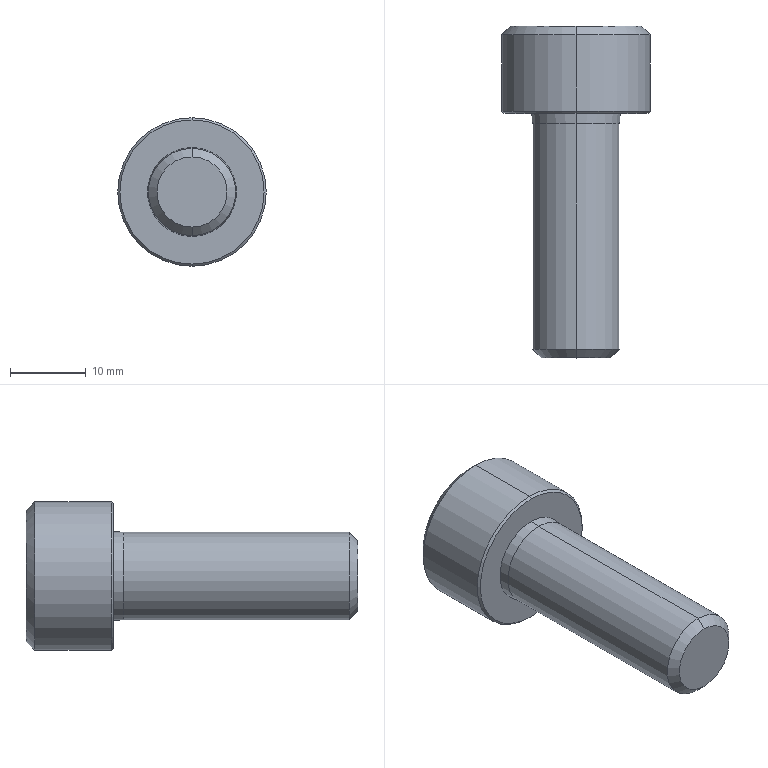Part | SolidWorks | features BaseBody 1 | 1 solid | 35 faces | box 19.615 x 43.846 x 19.615 mm | volume 6315 mm3 | cone 16 | plane 15 | cylinder 4 | commonest cylinder face diameters 11.538 x2 19.615 x2
STEP:
#1=CARTESIAN_POINT('',(-58.138,245.555,113.462));
#2=VERTEX_POINT('',#1);
#3=CARTESIAN_POINT('',(-58.138,245.555,101.923));
#4=VERTEX_POINT('',#3);
#5=CARTESIAN_POINT('',(-58.138,245.555,107.692));
#6=DIRECTION('',(0.,1.,0.));
#7=DIRECTION('',(0.,0.,1.));
#8=AXIS2_PLACEMENT_3D('',#5,#6,#7);
#9=CIRCLE('',#8,5.769);
#10=EDGE_CURVE('',#2,#4,#9,.T.);
#11=ORIENTED_EDGE('',*,*,#10,.T.);
#12=CARTESIAN_POINT('',(-58.138,275.346,101.923));
#13=VERTEX_POINT('',#12);
#14=CARTESIAN_POINT('',(-58.138,244.423,101.923));
#15=DIRECTION('',(0.,1.,0.));
#16=VECTOR('',#15,1000.);
#17=LINE('',#14,#16);
#18=EDGE_CURVE('',#4,#13,#17,.T.);
#19=ORIENTED_EDGE('',*,*,#18,.T.);
#20=CARTESIAN_POINT('',(-58.138,275.346,113.462));
#21=VERTEX_POINT('',#20);
#22=CARTESIAN_POINT('',(-58.138,275.346,107.692));
#23=DIRECTION('',(0.,-1.,0.));
#24=DIRECTION('',(0.,0.,1.));
#25=AXIS2_PLACEMENT_3D('',#22,#23,#24);
#26=CIRCLE('',#25,5.769);
#27=EDGE_CURVE('',#13,#21,#26,.T.);
#28=ORIENTED_EDGE('',*,*,#27,.T.);
#29=CARTESIAN_POINT('',(-58.138,244.423,113.462));
#30=DIRECTION('',(0.,1.,0.));
#31=VECTOR('',#30,1000.);
#32=LINE('',#29,#31);
#33=EDGE_CURVE('',#2,#21,#32,.T.);
#34=ORIENTED_EDGE('',*,*,#33,.F.);
#35=EDGE_LOOP('',(#11,#19,#28,#34));
#36=FACE_OUTER_BOUND('',#35,.T.);
#37=CARTESIAN_POINT('',(-58.138,244.423,107.692));
#38=DIRECTION('',(0.,1.,0.));
#39=DIRECTION('',(0.,0.,1.));
#40=AXIS2_PLACEMENT_3D('',#37,#38,#39);
#41=CYLINDRICAL_SURFACE('',#40,5.769);
#42=ADVANCED_FACE('',(#36),#41,.T.);
#43=ORIENTED_EDGE('',*,*,#27,.F.);
#44=CARTESIAN_POINT('',(-58.138,276.731,101.808));
#45=VERTEX_POINT('',#44);
#46=CARTESIAN_POINT('',(-58.138,276.731,101.808));
#47=DIRECTION('',(0.,0.9965,-0.08305));
#48=VECTOR('',#47,1000.);
#49=LINE('',#46,#48);
#50=EDGE_CURVE('',#13,#45,#49,.T.);
#51=ORIENTED_EDGE('',*,*,#50,.T.);
#52=CARTESIAN_POINT('',(-58.138,276.731,113.577));
#53=VERTEX_POINT('',#52);
#54=CARTESIAN_POINT('',(-58.138,276.731,107.692));
#55=DIRECTION('',(0.,-1.,0.));
#56=DIRECTION('',(0.,0.,1.));
#57=AXIS2_PLACEMENT_3D('',#54,#55,#56);
#58=CIRCLE('',#57,5.885);
#59=EDGE_CURVE('',#45,#53,#58,.T.);
#60=ORIENTED_EDGE('',*,*,#59,.T.);
#61=CARTESIAN_POINT('',(-58.138,276.731,113.577));
#62=DIRECTION('',(0.,0.9965,0.08305));
#63=VECTOR('',#62,1000.);
#64=LINE('',#61,#63);
#65=EDGE_CURVE('',#21,#53,#64,.T.);
#66=ORIENTED_EDGE('',*,*,#65,.F.);
#67=EDGE_LOOP('',(#43,#51,#60,#66));
#68=FACE_OUTER_BOUND('',#67,.T.);
#69=CARTESIAN_POINT('',(-58.138,276.731,107.692));
#70=DIRECTION('',(0.,1.,0.));
#71=DIRECTION('',(0.,0.,1.));
#72=AXIS2_PLACEMENT_3D('',#69,#70,#71);
#73=CONICAL_SURFACE('',#72,5.885,0.08314);
#74=ADVANCED_FACE('',(#68),#73,.T.);
#75=CARTESIAN_POINT('',(-58.138,244.423,112.33));
#76=VERTEX_POINT('',#75);
#77=CARTESIAN_POINT('',(-58.138,244.423,103.055));
#78=VERTEX_POINT('',#77);
#79=CARTESIAN_POINT('',(-58.138,244.423,107.692));
#80=DIRECTION('',(0.,1.,0.));
#81=DIRECTION('',(0.,0.,1.));
#82=AXIS2_PLACEMENT_3D('',#79,#80,#81);
#83=CIRCLE('',#82,4.637);
#84=EDGE_CURVE('',#76,#78,#83,.T.);
#85=ORIENTED_EDGE('',*,*,#84,.T.);
#86=CARTESIAN_POINT('',(-58.138,245.555,101.923));
#87=DIRECTION('',(0.,0.7071,-0.7071));
#88=VECTOR('',#87,1000.);
#89=LINE('',#86,#88);
#90=EDGE_CURVE('',#78,#4,#89,.T.);
#91=ORIENTED_EDGE('',*,*,#90,.T.);
#92=ORIENTED_EDGE('',*,*,#10,.F.);
#93=CARTESIAN_POINT('',(-58.138,245.555,113.462));
#94=DIRECTION('',(0.,0.7071,0.7071));
#95=VECTOR('',#94,1000.);
#96=LINE('',#93,#95);
#97=EDGE_CURVE('',#76,#2,#96,.T.);
#98=ORIENTED_EDGE('',*,*,#97,.F.);
#99=EDGE_LOOP('',(#85,#91,#92,#98));
#100=FACE_OUTER_BOUND('',#99,.T.);
#101=CARTESIAN_POINT('',(-58.138,245.555,107.692));
#102=DIRECTION('',(0.,1.,0.));
#103=DIRECTION('',(0.,0.,1.));
#104=AXIS2_PLACEMENT_3D('',#101,#102,#103);
#105=CONICAL_SURFACE('',#104,5.769,0.7854);
#106=ADVANCED_FACE('',(#100),#105,.T.);
#107=CARTESIAN_POINT('',(-58.138,276.731,117.212));
#108=VERTEX_POINT('',#107);
#109=CARTESIAN_POINT('',(-58.138,276.731,98.173));
#110=VERTEX_POINT('',#109);
#111=CARTESIAN_POINT('',(-58.138,276.731,107.692));
#112=DIRECTION('',(0.,1.,0.));
#113=DIRECTION('',(0.,0.,1.));
#114=AXIS2_PLACEMENT_3D('',#111,#112,#113);
#115=CIRCLE('',#114,9.519);
#116=EDGE_CURVE('',#108,#110,#115,.T.);
#117=ORIENTED_EDGE('',*,*,#116,.T.);
#118=CARTESIAN_POINT('',(-58.138,277.019,97.885));
#119=VERTEX_POINT('',#118);
#120=CARTESIAN_POINT('',(-58.138,277.019,97.885));
#121=DIRECTION('',(0.,0.7071,-0.7071));
#122=VECTOR('',#121,1000.);
#123=LINE('',#120,#122);
#124=EDGE_CURVE('',#110,#119,#123,.T.);
#125=ORIENTED_EDGE('',*,*,#124,.T.);
#126=CARTESIAN_POINT('',(-58.138,277.019,117.5));
#127=VERTEX_POINT('',#126);
#128=CARTESIAN_POINT('',(-58.138,277.019,107.692));
#129=DIRECTION('',(0.,-1.,0.));
#130=DIRECTION('',(-1.,0.,0.));
#131=AXIS2_PLACEMENT_3D('',#128,#129,#130);
#132=CIRCLE('',#131,9.808);
#133=EDGE_CURVE('',#119,#127,#132,.T.);
#134=ORIENTED_EDGE('',*,*,#133,.T.);
#135=CARTESIAN_POINT('',(-58.138,277.019,117.5));
#136=DIRECTION('',(0.,0.7071,0.7071));
#137=VECTOR('',#136,1000.);
#138=LINE('',#135,#137);
#139=EDGE_CURVE('',#108,#127,#138,.T.);
#140=ORIENTED_EDGE('',*,*,#139,.F.);
#141=EDGE_LOOP('',(#117,#125,#134,#140));
#142=FACE_OUTER_BOUND('',#141,.T.);
#143=CARTESIAN_POINT('',(-58.138,277.019,107.692));
#144=DIRECTION('',(0.,1.,0.));
#145=DIRECTION('',(0.,0.,1.));
#146=AXIS2_PLACEMENT_3D('',#143,#144,#145);
#147=CONICAL_SURFACE('',#146,9.808,0.7854);
#148=ADVANCED_FACE('',(#142),#147,.T.);
#149=ORIENTED_EDGE('',*,*,#133,.F.);
#150=CARTESIAN_POINT('',(-58.138,287.115,97.885));
#151=VERTEX_POINT('',#150);
#152=CARTESIAN_POINT('',(-58.138,244.423,97.885));
#153=DIRECTION('',(0.,1.,0.));
#154=VECTOR('',#153,1000.);
#155=LINE('',#152,#154);
#156=EDGE_CURVE('',#119,#151,#155,.T.);
#157=ORIENTED_EDGE('',*,*,#156,.T.);
#158=CARTESIAN_POINT('',(-58.138,287.115,117.5));
#159=VERTEX_POINT('',#158);
#160=CARTESIAN_POINT('',(-58.138,287.115,107.692));
#161=DIRECTION('',(0.,-1.,0.));
#162=DIRECTION('',(0.,0.,1.));
#163=AXIS2_PLACEMENT_3D('',#160,#161,#162);
#164=CIRCLE('',#163,9.808);
#165=EDGE_CURVE('',#151,#159,#164,.T.);
#166=ORIENTED_EDGE('',*,*,#165,.T.);
#167=CARTESIAN_POINT('',(-58.138,244.423,117.5));
#168=DIRECTION('',(0.,1.,0.));
#169=VECTOR('',#168,1000.);
#170=LINE('',#167,#169);
#171=EDGE_CURVE('',#127,#159,#170,.T.);
#172=ORIENTED_EDGE('',*,*,#171,.F.);
#173=EDGE_LOOP('',(#149,#157,#166,#172));
#174=FACE_OUTER_BOUND('',#173,.T.);
#175=CARTESIAN_POINT('',(-58.138,244.423,107.692));
#176=DIRECTION('',(0.,1.,0.));
#177=DIRECTION('',(0.,0.,1.));
#178=AXIS2_PLACEMENT_3D('',#175,#176,#177);
#179=CYLINDRICAL_SURFACE('',#178,9.808);
#180=ADVANCED_FACE('',(#174),#179,.T.);
#181=CARTESIAN_POINT('',(-58.138,288.269,99.038));
#182=VERTEX_POINT('',#181);
#183=CARTESIAN_POINT('',(-58.138,288.269,116.346));
#184=VERTEX_POINT('',#183);
#185=CARTESIAN_POINT('',(-58.138,288.269,107.692));
#186=DIRECTION('',(0.,-1.,0.));
#187=DIRECTION('',(0.,0.,-1.));
#188=AXIS2_PLACEMENT_3D('',#185,#186,#187);
#189=CIRCLE('',#188,8.654);
#190=EDGE_CURVE('',#182,#184,#189,.T.);
#191=ORIENTED_EDGE('',*,*,#190,.T.);
#192=CARTESIAN_POINT('',(-58.138,287.115,117.5));
#193=DIRECTION('',(0.,-0.7071,0.7071));
#194=VECTOR('',#193,1000.);
#195=LINE('',#192,#194);
#196=EDGE_CURVE('',#184,#159,#195,.T.);
#197=ORIENTED_EDGE('',*,*,#196,.T.);
#198=ORIENTED_EDGE('',*,*,#165,.F.);
#199=CARTESIAN_POINT('',(-58.138,287.115,97.885));
#200=DIRECTION('',(0.,-0.7071,-0.7071));
#201=VECTOR('',#200,1000.);
#202=LINE('',#199,#201);
#203=EDGE_CURVE('',#182,#151,#202,.T.);
#204=ORIENTED_EDGE('',*,*,#203,.F.);
#205=EDGE_LOOP('',(#191,#197,#198,#204));
#206=FACE_OUTER_BOUND('',#205,.T.);
#207=CARTESIAN_POINT('',(-58.138,287.115,107.692));
#208=DIRECTION('',(0.,-1.,0.));
#209=DIRECTION('',(0.,0.,-1.));
#210=AXIS2_PLACEMENT_3D('',#207,#208,#209);
#211=CONICAL_SURFACE('',#210,9.808,0.7854);
#212=ADVANCED_FACE('',(#206),#211,.T.);
#213=CARTESIAN_POINT('',(-58.138,279.835,107.692));
#214=VERTEX_POINT('',#213);
#215=CARTESIAN_POINT('',(-58.138,282.5,112.308));
#216=VERTEX_POINT('',#215);
#217=CARTESIAN_POINT('',(-58.138,282.5,112.308));
#218=DIRECTION('',(0.,0.5,0.866));
#219=VECTOR('',#218,1000.);
#220=LINE('',#217,#219);
#221=EDGE_CURVE('',#214,#216,#220,.T.);
#222=ORIENTED_EDGE('',*,*,#221,.F.);
#223=CARTESIAN_POINT('',(-58.138,282.5,103.077));
#224=VERTEX_POINT('',#223);
#225=CARTESIAN_POINT('',(-58.138,282.5,103.077));
#226=DIRECTION('',(0.,0.5,-0.866));
#227=VECTOR('',#226,1000.);
#228=LINE('',#225,#227);
#229=EDGE_CURVE('',#214,#224,#228,.T.);
#230=ORIENTED_EDGE('',*,*,#229,.T.);
#231=CARTESIAN_POINT('',(-60.446,282.5,103.695));
#232=VERTEX_POINT('',#231);
#233=CARTESIAN_POINT('',(-58.138,282.5,107.692));
#234=DIRECTION('',(0.,-1.,0.));
#235=DIRECTION('',(0.,0.,1.));
#236=AXIS2_PLACEMENT_3D('',#233,#234,#235);
#237=CIRCLE('',#236,4.615);
#238=EDGE_CURVE('',#232,#224,#237,.T.);
#239=ORIENTED_EDGE('',*,*,#238,.F.);
#240=CARTESIAN_POINT('',(-62.753,282.5,107.692));
#241=VERTEX_POINT('',#240);
#242=CARTESIAN_POINT('',(-58.138,282.5,107.692));
#243=DIRECTION('',(0.,-1.,0.));
#244=DIRECTION('',(0.,0.,1.));
#245=AXIS2_PLACEMENT_3D('',#242,#243,#244);
#246=CIRCLE('',#245,4.615);
#247=EDGE_CURVE('',#241,#232,#246,.T.);
#248=ORIENTED_EDGE('',*,*,#247,.F.);
#249=CARTESIAN_POINT('',(-60.446,282.5,111.689));
#250=VERTEX_POINT('',#249);
#251=CARTESIAN_POINT('',(-58.138,282.5,107.692));
#252=DIRECTION('',(0.,-1.,0.));
#253=DIRECTION('',(0.,0.,1.));
#254=AXIS2_PLACEMENT_3D('',#251,#252,#253);
#255=CIRCLE('',#254,4.615);
#256=EDGE_CURVE('',#250,#241,#255,.T.);
#257=ORIENTED_EDGE('',*,*,#256,.F.);
#258=CARTESIAN_POINT('',(-58.138,282.5,107.692));
#259=DIRECTION('',(0.,-1.,0.));
#260=DIRECTION('',(0.,0.,1.));
#261=AXIS2_PLACEMENT_3D('',#258,#259,#260);
#262=CIRCLE('',#261,4.615);
#263=EDGE_CURVE('',#216,#250,#262,.T.);
#264=ORIENTED_EDGE('',*,*,#263,.F.);
#265=EDGE_LOOP('',(#222,#230,#239,#248,#257,#264));
#266=FACE_OUTER_BOUND('',#265,.T.);
#267=CARTESIAN_POINT('',(-58.138,282.5,107.692));
#268=DIRECTION('',(0.,1.,0.));
#269=DIRECTION('',(0.,0.,1.));
#270=AXIS2_PLACEMENT_3D('',#267,#268,#269);
#271=CONICAL_SURFACE('',#270,4.615,1.047);
#272=ADVANCED_FACE('',(#266),#271,.F.);
#273=ORIENTED_EDGE('',*,*,#18,.F.);
#274=CARTESIAN_POINT('',(-58.138,245.555,107.692));
#275=DIRECTION('',(0.,1.,0.));
#276=DIRECTION('',(0.,0.,1.));
#277=AXIS2_PLACEMENT_3D('',#274,#275,#276);
#278=CIRCLE('',#277,5.769);
#279=EDGE_CURVE('',#4,#2,#278,.T.);
#280=ORIENTED_EDGE('',*,*,#279,.T.);
#281=ORIENTED_EDGE('',*,*,#33,.T.);
#282=CARTESIAN_POINT('',(-58.138,275.346,107.692));
#283=DIRECTION('',(0.,-1.,0.));
#284=DIRECTION('',(0.,0.,1.));
#285=AXIS2_PLACEMENT_3D('',#282,#283,#284);
#286=CIRCLE('',#285,5.769);
#287=EDGE_CURVE('',#21,#13,#286,.T.);
#288=ORIENTED_EDGE('',*,*,#287,.T.);
#289=EDGE_LOOP('',(#273,#280,#281,#288));
#290=FACE_OUTER_BOUND('',#289,.T.);
#291=CARTESIAN_POINT('',(-58.138,244.423,107.692));
#292=DIRECTION('',(0.,1.,0.));
#293=DIRECTION('',(0.,0.,1.));
#294=AXIS2_PLACEMENT_3D('',#291,#292,#293);
#295=CYLINDRICAL_SURFACE('',#294,5.769);
#296=ADVANCED_FACE('',(#290),#295,.T.);
#297=ORIENTED_EDGE('',*,*,#50,.F.);
#298=ORIENTED_EDGE('',*,*,#287,.F.);
#299=ORIENTED_EDGE('',*,*,#65,.T.);
#300=CARTESIAN_POINT('',(-58.138,276.731,107.692));
#301=DIRECTION('',(0.,-1.,0.));
#302=DIRECTION('',(0.,0.,1.));
#303=AXIS2_PLACEMENT_3D('',#300,#301,#302);
#304=CIRCLE('',#303,5.885);
#305=EDGE_CURVE('',#53,#45,#304,.T.);
#306=ORIENTED_EDGE('',*,*,#305,.T.);
#307=EDGE_LOOP('',(#297,#298,#299,#306));
#308=FACE_OUTER_BOUND('',#307,.T.);
#309=CARTESIAN_POINT('',(-58.138,276.731,107.692));
#310=DIRECTION('',(0.,1.,0.));
#311=DIRECTION('',(0.,0.,1.));
#312=AXIS2_PLACEMENT_3D('',#309,#310,#311);
#313=CONICAL_SURFACE('',#312,5.885,0.08314);
#314=ADVANCED_FACE('',(#308),#313,.T.);
#315=ORIENTED_EDGE('',*,*,#90,.F.);
#316=CARTESIAN_POINT('',(-58.138,244.423,107.692));
#317=DIRECTION('',(0.,1.,0.));
#318=DIRECTION('',(0.,0.,1.));
#319=AXIS2_PLACEMENT_3D('',#316,#317,#318);
#320=CIRCLE('',#319,4.637);
#321=EDGE_CURVE('',#78,#76,#320,.T.);
#322=ORIENTED_EDGE('',*,*,#321,.T.);
#323=ORIENTED_EDGE('',*,*,#97,.T.);
#324=ORIENTED_EDGE('',*,*,#279,.F.);
#325=EDGE_LOOP('',(#315,#322,#323,#324));
#326=FACE_OUTER_BOUND('',#325,.T.);
#327=CARTESIAN_POINT('',(-58.138,245.555,107.692));
#328=DIRECTION('',(0.,1.,0.));
#329=DIRECTION('',(0.,0.,1.));
#330=AXIS2_PLACEMENT_3D('',#327,#328,#329);
#331=CONICAL_SURFACE('',#330,5.769,0.7854);
#332=ADVANCED_FACE('',(#326),#331,.T.);
#333=ORIENTED_EDGE('',*,*,#305,.F.);
#334=ORIENTED_EDGE('',*,*,#59,.F.);
#335=EDGE_LOOP('',(#333,#334));
#336=FACE_BOUND('',#335,.T.);
#337=ORIENTED_EDGE('',*,*,#116,.F.);
#338=CARTESIAN_POINT('',(-58.138,276.731,107.692));
#339=DIRECTION('',(0.,1.,0.));
#340=DIRECTION('',(0.,0.,1.));
#341=AXIS2_PLACEMENT_3D('',#338,#339,#340);
#342=CIRCLE('',#341,9.519);
#343=EDGE_CURVE('',#110,#108,#342,.T.);
#344=ORIENTED_EDGE('',*,*,#343,.F.);
#345=EDGE_LOOP('',(#337,#344));
#346=FACE_OUTER_BOUND('',#345,.T.);
#347=CARTESIAN_POINT('',(-67.657,276.731,107.692));
#348=DIRECTION('',(0.,1.,0.));
#349=DIRECTION('',(0.,0.,1.));
#350=AXIS2_PLACEMENT_3D('',#347,#348,#349);
#351=PLANE('',#350);
#352=ADVANCED_FACE('',(#336,#346),#351,.F.);
#353=ORIENTED_EDGE('',*,*,#84,.F.);
#354=ORIENTED_EDGE('',*,*,#321,.F.);
#355=EDGE_LOOP('',(#353,#354));
#356=FACE_OUTER_BOUND('',#355,.T.);
#357=CARTESIAN_POINT('',(-62.775,244.423,107.692));
#358=DIRECTION('',(0.,1.,0.));
#359=DIRECTION('',(0.,0.,1.));
#360=AXIS2_PLACEMENT_3D('',#357,#358,#359);
#361=PLANE('',#360);
#362=ADVANCED_FACE('',(#356),#361,.F.);
#363=ORIENTED_EDGE('',*,*,#124,.F.);
#364=ORIENTED_EDGE('',*,*,#343,.T.);
#365=ORIENTED_EDGE('',*,*,#139,.T.);
#366=CARTESIAN_POINT('',(-58.138,277.019,107.692));
#367=DIRECTION('',(0.,-1.,0.));
#368=DIRECTION('',(-1.,0.,0.));
#369=AXIS2_PLACEMENT_3D('',#366,#367,#368);
#370=CIRCLE('',#369,9.808);
#371=EDGE_CURVE('',#127,#119,#370,.T.);
#372=ORIENTED_EDGE('',*,*,#371,.T.);
#373=EDGE_LOOP('',(#363,#364,#365,#372));
#374=FACE_OUTER_BOUND('',#373,.T.);
#375=CARTESIAN_POINT('',(-58.138,277.019,107.692));
#376=DIRECTION('',(0.,1.,0.));
#377=DIRECTION('',(0.,0.,1.));
#378=AXIS2_PLACEMENT_3D('',#375,#376,#377);
#379=CONICAL_SURFACE('',#378,9.808,0.7854);
#380=ADVANCED_FACE('',(#374),#379,.T.);
#381=ORIENTED_EDGE('',*,*,#156,.F.);
#382=ORIENTED_EDGE('',*,*,#371,.F.);
#383=ORIENTED_EDGE('',*,*,#171,.T.);
#384=CARTESIAN_POINT('',(-58.138,287.115,107.692));
#385=DIRECTION('',(0.,-1.,0.));
#386=DIRECTION('',(0.,0.,1.));
#387=AXIS2_PLACEMENT_3D('',#384,#385,#386);
#388=CIRCLE('',#387,9.808);
#389=EDGE_CURVE('',#159,#151,#388,.T.);
#390=ORIENTED_EDGE('',*,*,#389,.T.);
#391=EDGE_LOOP('',(#381,#382,#383,#390));
#392=FACE_OUTER_BOUND('',#391,.T.);
#393=CARTESIAN_POINT('',(-58.138,244.423,107.692));
#394=DIRECTION('',(0.,1.,0.));
#395=DIRECTION('',(0.,0.,1.));
#396=AXIS2_PLACEMENT_3D('',#393,#394,#395);
#397=CYLINDRICAL_SURFACE('',#396,9.808);
#398=ADVANCED_FACE('',(#392),#397,.T.);
#399=ORIENTED_EDGE('',*,*,#196,.F.);
#400=CARTESIAN_POINT('',(-58.138,288.269,107.692));
#401=DIRECTION('',(0.,-1.,0.));
#402=DIRECTION('',(0.,0.,-1.));
#403=AXIS2_PLACEMENT_3D('',#400,#401,#402);
#404=CIRCLE('',#403,8.654);
#405=EDGE_CURVE('',#184,#182,#404,.T.);
#406=ORIENTED_EDGE('',*,*,#405,.T.);
#407=ORIENTED_EDGE('',*,*,#203,.T.);
#408=ORIENTED_EDGE('',*,*,#389,.F.);
#409=EDGE_LOOP('',(#399,#406,#407,#408));
#410=FACE_OUTER_BOUND('',#409,.T.);
#411=CARTESIAN_POINT('',(-58.138,287.115,107.692));
#412=DIRECTION('',(0.,-1.,0.));
#413=DIRECTION('',(0.,0.,-1.));
#414=AXIS2_PLACEMENT_3D('',#411,#412,#413);
#415=CONICAL_SURFACE('',#414,9.808,0.7854);
#416=ADVANCED_FACE('',(#410),#415,.T.);
#417=CARTESIAN_POINT('',(-53.523,288.269,105.028));
#418=VERTEX_POINT('',#417);
#419=CARTESIAN_POINT('',(-58.138,288.269,102.363));
#420=VERTEX_POINT('',#419);
#421=CARTESIAN_POINT('',(-58.138,288.269,107.692));
#422=DIRECTION('',(0.,1.,0.));
#423=DIRECTION('',(0.,0.,1.));
#424=AXIS2_PLACEMENT_3D('',#421,#422,#423);
#425=CIRCLE('',#424,5.329);
#426=EDGE_CURVE('',#418,#420,#425,.T.);
#427=ORIENTED_EDGE('',*,*,#426,.F.);
#428=CARTESIAN_POINT('',(-53.523,288.269,110.357));
#429=VERTEX_POINT('',#428);
#430=CARTESIAN_POINT('',(-58.138,288.269,107.692));
#431=DIRECTION('',(0.,1.,0.));
#432=DIRECTION('',(0.,0.,1.));
#433=AXIS2_PLACEMENT_3D('',#430,#431,#432);
#434=CIRCLE('',#433,5.329);
#435=EDGE_CURVE('',#429,#418,#434,.T.);
#436=ORIENTED_EDGE('',*,*,#435,.F.);
#437=CARTESIAN_POINT('',(-58.138,288.269,113.022));
#438=VERTEX_POINT('',#437);
#439=CARTESIAN_POINT('',(-58.138,288.269,107.692));
#440=DIRECTION('',(0.,1.,0.));
#441=DIRECTION('',(0.,0.,1.));
#442=AXIS2_PLACEMENT_3D('',#439,#440,#441);
#443=CIRCLE('',#442,5.329);
#444=EDGE_CURVE('',#438,#429,#443,.T.);
#445=ORIENTED_EDGE('',*,*,#444,.F.);
#446=CARTESIAN_POINT('',(-62.753,288.269,110.357));
#447=VERTEX_POINT('',#446);
#448=CARTESIAN_POINT('',(-58.138,288.269,107.692));
#449=DIRECTION('',(0.,1.,0.));
#450=DIRECTION('',(0.,0.,1.));
#451=AXIS2_PLACEMENT_3D('',#448,#449,#450);
#452=CIRCLE('',#451,5.329);
#453=EDGE_CURVE('',#447,#438,#452,.T.);
#454=ORIENTED_EDGE('',*,*,#453,.F.);
#455=CARTESIAN_POINT('',(-62.753,288.269,105.028));
#456=VERTEX_POINT('',#455);
#457=CARTESIAN_POINT('',(-58.138,288.269,107.692));
#458=DIRECTION('',(0.,1.,0.));
#459=DIRECTION('',(0.,0.,1.));
#460=AXIS2_PLACEMENT_3D('',#457,#458,#459);
#461=CIRCLE('',#460,5.329);
#462=EDGE_CURVE('',#456,#447,#461,.T.);
#463=ORIENTED_EDGE('',*,*,#462,.F.);
#464=CARTESIAN_POINT('',(-58.138,288.269,107.692));
#465=DIRECTION('',(0.,1.,0.));
#466=DIRECTION('',(0.,0.,1.));
#467=AXIS2_PLACEMENT_3D('',#464,#465,#466);
#468=CIRCLE('',#467,5.329);
#469=EDGE_CURVE('',#420,#456,#468,.T.);
#470=ORIENTED_EDGE('',*,*,#469,.F.);
#471=EDGE_LOOP('',(#427,#436,#445,#454,#463,#470));
#472=FACE_BOUND('',#471,.T.);
#473=ORIENTED_EDGE('',*,*,#190,.F.);
#474=ORIENTED_EDGE('',*,*,#405,.F.);
#475=EDGE_LOOP('',(#473,#474));
#476=FACE_OUTER_BOUND('',#475,.T.);
#477=CARTESIAN_POINT('',(-63.467,288.269,107.692));
#478=DIRECTION('',(0.,-1.,0.));
#479=DIRECTION('',(0.,0.,-1.));
#480=AXIS2_PLACEMENT_3D('',#477,#478,#479);
#481=PLANE('',#480);
#482=ADVANCED_FACE('',(#472,#476),#481,.F.);
#483=CARTESIAN_POINT('',(-58.138,288.269,102.363));
#484=CARTESIAN_POINT('',(-58.499,288.061,102.571));
#485=CARTESIAN_POINT('',(-58.867,287.884,102.784));
#486=CARTESIAN_POINT('',(-59.44,287.694,103.115));
#487=CARTESIAN_POINT('',(-59.635,287.644,103.227));
#488=CARTESIAN_POINT('',(-60.031,287.574,103.456));
#489=CARTESIAN_POINT('',(-60.236,287.556,103.574));
#490=CARTESIAN_POINT('',(-60.84,287.554,103.923));
#491=CARTESIAN_POINT('',(-61.236,287.625,104.152));
#492=CARTESIAN_POINT('',(-62.017,287.88,104.603));
#493=CARTESIAN_POINT('',(-62.391,288.06,104.818));
#494=CARTESIAN_POINT('',(-62.753,288.269,105.028));
#495=B_SPLINE_CURVE_WITH_KNOTS('',3,(#483,#484,#485,#486,#487,#488,#489,#490,#491,#492,#493,#494),.UNSPECIFIED.,.F.,.F.,(4,2,2,2,2,4),(0.,0.001376,0.002064,0.002753,0.004129,0.005505),.UNSPECIFIED.);
#496=EDGE_CURVE('',#420,#456,#495,.T.);
#497=ORIENTED_EDGE('',*,*,#496,.F.);
#498=ORIENTED_EDGE('',*,*,#469,.T.);
#499=EDGE_LOOP('',(#497,#498));
#500=FACE_OUTER_BOUND('',#499,.T.);
#501=CARTESIAN_POINT('',(-58.138,288.269,107.692));
#502=DIRECTION('',(0.,1.,0.));
#503=DIRECTION('',(0.,0.,1.));
#504=AXIS2_PLACEMENT_3D('',#501,#502,#503);
#505=CONICAL_SURFACE('',#504,5.329,0.7854);
#506=ADVANCED_FACE('',(#500),#505,.F.);
#507=CARTESIAN_POINT('',(-53.523,288.269,105.028));
#508=CARTESIAN_POINT('',(-53.883,288.061,104.819));
#509=CARTESIAN_POINT('',(-54.252,287.884,104.607));
#510=CARTESIAN_POINT('',(-54.825,287.694,104.276));
#511=CARTESIAN_POINT('',(-55.019,287.644,104.164));
#512=CARTESIAN_POINT('',(-55.416,287.574,103.934));
#513=CARTESIAN_POINT('',(-55.62,287.556,103.816));
#514=CARTESIAN_POINT('',(-56.225,287.554,103.468));
#515=CARTESIAN_POINT('',(-56.621,287.625,103.239));
#516=CARTESIAN_POINT('',(-57.402,287.88,102.788));
#517=CARTESIAN_POINT('',(-57.775,288.06,102.572));
#518=CARTESIAN_POINT('',(-58.138,288.269,102.363));
#519=B_SPLINE_CURVE_WITH_KNOTS('',3,(#507,#508,#509,#510,#511,#512,#513,#514,#515,#516,#517,#518),.UNSPECIFIED.,.F.,.F.,(4,2,2,2,2,4),(0.,0.001376,0.002064,0.002753,0.004129,0.005505),.UNSPECIFIED.);
#520=EDGE_CURVE('',#418,#420,#519,.T.);
#521=ORIENTED_EDGE('',*,*,#520,.F.);
#522=ORIENTED_EDGE('',*,*,#426,.T.);
#523=EDGE_LOOP('',(#521,#522));
#524=FACE_OUTER_BOUND('',#523,.T.);
#525=CARTESIAN_POINT('',(-58.138,288.269,107.692));
#526=DIRECTION('',(0.,1.,0.));
#527=DIRECTION('',(0.,0.,1.));
#528=AXIS2_PLACEMENT_3D('',#525,#526,#527);
#529=CONICAL_SURFACE('',#528,5.329,0.7854);
#530=ADVANCED_FACE('',(#524),#529,.F.);
#531=CARTESIAN_POINT('',(-53.523,288.269,110.357));
#532=CARTESIAN_POINT('',(-53.523,288.061,109.941));
#533=CARTESIAN_POINT('',(-53.523,287.884,109.515));
#534=CARTESIAN_POINT('',(-53.523,287.694,108.853));
#535=CARTESIAN_POINT('',(-53.523,287.644,108.629));
#536=CARTESIAN_POINT('',(-53.523,287.574,108.171));
#537=CARTESIAN_POINT('',(-53.523,287.556,107.935));
#538=CARTESIAN_POINT('',(-53.523,287.554,107.237));
#539=CARTESIAN_POINT('',(-53.523,287.625,106.78));
#540=CARTESIAN_POINT('',(-53.523,287.88,105.878));
#541=CARTESIAN_POINT('',(-53.523,288.06,105.446));
#542=CARTESIAN_POINT('',(-53.523,288.269,105.028));
#543=B_SPLINE_CURVE_WITH_KNOTS('',3,(#531,#532,#533,#534,#535,#536,#537,#538,#539,#540,#541,#542),.UNSPECIFIED.,.F.,.F.,(4,2,2,2,2,4),(0.,0.001376,0.002064,0.002753,0.004129,0.005505),.UNSPECIFIED.);
#544=EDGE_CURVE('',#429,#418,#543,.T.);
#545=ORIENTED_EDGE('',*,*,#544,.F.);
#546=ORIENTED_EDGE('',*,*,#435,.T.);
#547=EDGE_LOOP('',(#545,#546));
#548=FACE_OUTER_BOUND('',#547,.T.);
#549=CARTESIAN_POINT('',(-58.138,288.269,107.692));
#550=DIRECTION('',(0.,1.,0.));
#551=DIRECTION('',(0.,0.,1.));
#552=AXIS2_PLACEMENT_3D('',#549,#550,#551);
#553=CONICAL_SURFACE('',#552,5.329,0.7854);
#554=ADVANCED_FACE('',(#548),#553,.F.);
#555=CARTESIAN_POINT('',(-58.138,288.269,113.022));
#556=CARTESIAN_POINT('',(-57.777,288.061,112.813));
#557=CARTESIAN_POINT('',(-57.409,287.884,112.601));
#558=CARTESIAN_POINT('',(-56.836,287.694,112.27));
#559=CARTESIAN_POINT('',(-56.642,287.644,112.158));
#560=CARTESIAN_POINT('',(-56.245,287.574,111.929));
#561=CARTESIAN_POINT('',(-56.04,287.556,111.811));
#562=CARTESIAN_POINT('',(-55.436,287.554,111.462));
#563=CARTESIAN_POINT('',(-55.04,287.625,111.233));
#564=CARTESIAN_POINT('',(-54.259,287.88,110.782));
#565=CARTESIAN_POINT('',(-53.885,288.06,110.566));
#566=CARTESIAN_POINT('',(-53.523,288.269,110.357));
#567=B_SPLINE_CURVE_WITH_KNOTS('',3,(#555,#556,#557,#558,#559,#560,#561,#562,#563,#564,#565,#566),.UNSPECIFIED.,.F.,.F.,(4,2,2,2,2,4),(0.,0.001376,0.002064,0.002753,0.004129,0.005505),.UNSPECIFIED.);
#568=EDGE_CURVE('',#438,#429,#567,.T.);
#569=ORIENTED_EDGE('',*,*,#568,.F.);
#570=ORIENTED_EDGE('',*,*,#444,.T.);
#571=EDGE_LOOP('',(#569,#570));
#572=FACE_OUTER_BOUND('',#571,.T.);
#573=CARTESIAN_POINT('',(-58.138,288.269,107.692));
#574=DIRECTION('',(0.,1.,0.));
#575=DIRECTION('',(0.,0.,1.));
#576=AXIS2_PLACEMENT_3D('',#573,#574,#575);
#577=CONICAL_SURFACE('',#576,5.329,0.7854);
#578=ADVANCED_FACE('',(#572),#577,.F.);
#579=CARTESIAN_POINT('',(-62.753,288.269,110.357));
#580=CARTESIAN_POINT('',(-62.393,288.061,110.565));
#581=CARTESIAN_POINT('',(-62.024,287.884,110.778));
#582=CARTESIAN_POINT('',(-61.451,287.694,111.109));
#583=CARTESIAN_POINT('',(-61.257,287.644,111.221));
#584=CARTESIAN_POINT('',(-60.86,287.574,111.45));
#585=CARTESIAN_POINT('',(-60.656,287.556,111.568));
#586=CARTESIAN_POINT('',(-60.051,287.554,111.917));
#587=CARTESIAN_POINT('',(-59.655,287.625,112.146));
#588=CARTESIAN_POINT('',(-58.874,287.88,112.597));
#589=CARTESIAN_POINT('',(-58.501,288.06,112.812));
#590=CARTESIAN_POINT('',(-58.138,288.269,113.022));
#591=B_SPLINE_CURVE_WITH_KNOTS('',3,(#579,#580,#581,#582,#583,#584,#585,#586,#587,#588,#589,#590),.UNSPECIFIED.,.F.,.F.,(4,2,2,2,2,4),(0.,0.001376,0.002064,0.002753,0.004129,0.005505),.UNSPECIFIED.);
#592=EDGE_CURVE('',#447,#438,#591,.T.);
#593=ORIENTED_EDGE('',*,*,#592,.F.);
#594=ORIENTED_EDGE('',*,*,#453,.T.);
#595=EDGE_LOOP('',(#593,#594));
#596=FACE_OUTER_BOUND('',#595,.T.);
#597=CARTESIAN_POINT('',(-58.138,288.269,107.692));
#598=DIRECTION('',(0.,1.,0.));
#599=DIRECTION('',(0.,0.,1.));
#600=AXIS2_PLACEMENT_3D('',#597,#598,#599);
#601=CONICAL_SURFACE('',#600,5.329,0.7854);
#602=ADVANCED_FACE('',(#596),#601,.F.);
#603=CARTESIAN_POINT('',(-62.753,288.269,105.028));
#604=CARTESIAN_POINT('',(-62.753,288.061,105.444));
#605=CARTESIAN_POINT('',(-62.753,287.884,105.87));
#606=CARTESIAN_POINT('',(-62.753,287.694,106.531));
#607=CARTESIAN_POINT('',(-62.753,287.644,106.756));
#608=CARTESIAN_POINT('',(-62.753,287.574,107.214));
#609=CARTESIAN_POINT('',(-62.753,287.556,107.45));
#610=CARTESIAN_POINT('',(-62.753,287.554,108.148));
#611=CARTESIAN_POINT('',(-62.753,287.625,108.605));
#612=CARTESIAN_POINT('',(-62.753,287.88,109.507));
#613=CARTESIAN_POINT('',(-62.753,288.06,109.938));
#614=CARTESIAN_POINT('',(-62.753,288.269,110.357));
#615=B_SPLINE_CURVE_WITH_KNOTS('',3,(#603,#604,#605,#606,#607,#608,#609,#610,#611,#612,#613,#614),.UNSPECIFIED.,.F.,.F.,(4,2,2,2,2,4),(0.,0.001376,0.002064,0.002753,0.004129,0.005505),.UNSPECIFIED.);
#616=EDGE_CURVE('',#456,#447,#615,.T.);
#617=ORIENTED_EDGE('',*,*,#616,.F.);
#618=ORIENTED_EDGE('',*,*,#462,.T.);
#619=EDGE_LOOP('',(#617,#618));
#620=FACE_OUTER_BOUND('',#619,.T.);
#621=CARTESIAN_POINT('',(-58.138,288.269,107.692));
#622=DIRECTION('',(0.,1.,0.));
#623=DIRECTION('',(0.,0.,1.));
#624=AXIS2_PLACEMENT_3D('',#621,#622,#623);
#625=CONICAL_SURFACE('',#624,5.329,0.7854);
#626=ADVANCED_FACE('',(#620),#625,.F.);
#627=CARTESIAN_POINT('',(-62.753,282.5,105.028));
#628=VERTEX_POINT('',#627);
#629=CARTESIAN_POINT('',(-62.753,282.5,105.028));
#630=DIRECTION('',(0.,1.,0.));
#631=VECTOR('',#630,1000.);
#632=LINE('',#629,#631);
#633=EDGE_CURVE('',#628,#456,#632,.T.);
#634=ORIENTED_EDGE('',*,*,#633,.F.);
#635=CARTESIAN_POINT('',(-58.138,282.5,102.363));
#636=DIRECTION('',(-0.866,0.,0.5));
#637=VECTOR('',#636,1000.);
#638=LINE('',#635,#637);
#639=EDGE_CURVE('',#232,#628,#638,.T.);
#640=ORIENTED_EDGE('',*,*,#639,.F.);
#641=CARTESIAN_POINT('',(-58.138,282.5,102.363));
#642=VERTEX_POINT('',#641);
#643=CARTESIAN_POINT('',(-58.138,282.5,102.363));
#644=DIRECTION('',(-0.866,0.,0.5));
#645=VECTOR('',#644,1000.);
#646=LINE('',#643,#645);
#647=EDGE_CURVE('',#642,#232,#646,.T.);
#648=ORIENTED_EDGE('',*,*,#647,.F.);
#649=CARTESIAN_POINT('',(-58.138,282.5,102.363));
#650=DIRECTION('',(0.,-1.,0.));
#651=VECTOR('',#650,1000.);
#652=LINE('',#649,#651);
#653=EDGE_CURVE('',#420,#642,#652,.T.);
#654=ORIENTED_EDGE('',*,*,#653,.F.);
#655=ORIENTED_EDGE('',*,*,#496,.T.);
#656=EDGE_LOOP('',(#634,#640,#648,#654,#655));
#657=FACE_OUTER_BOUND('',#656,.T.);
#658=CARTESIAN_POINT('',(-58.138,282.5,102.363));
#659=DIRECTION('',(-0.5,0.,-0.866));
#660=DIRECTION('',(-0.866,0.,0.5));
#661=AXIS2_PLACEMENT_3D('',#658,#659,#660);
#662=PLANE('',#661);
#663=ADVANCED_FACE('',(#657),#662,.F.);
#664=ORIENTED_EDGE('',*,*,#653,.T.);
#665=CARTESIAN_POINT('',(-55.83,282.5,103.695));
#666=VERTEX_POINT('',#665);
#667=CARTESIAN_POINT('',(-53.523,282.5,105.028));
#668=DIRECTION('',(-0.866,0.,-0.5));
#669=VECTOR('',#668,1000.);
#670=LINE('',#667,#669);
#671=EDGE_CURVE('',#666,#642,#670,.T.);
#672=ORIENTED_EDGE('',*,*,#671,.F.);
#673=CARTESIAN_POINT('',(-53.523,282.5,105.028));
#674=VERTEX_POINT('',#673);
#675=CARTESIAN_POINT('',(-53.523,282.5,105.028));
#676=DIRECTION('',(-0.866,0.,-0.5));
#677=VECTOR('',#676,1000.);
#678=LINE('',#675,#677);
#679=EDGE_CURVE('',#674,#666,#678,.T.);
#680=ORIENTED_EDGE('',*,*,#679,.F.);
#681=CARTESIAN_POINT('',(-53.523,282.5,105.028));
#682=DIRECTION('',(0.,-1.,0.));
#683=VECTOR('',#682,1000.);
#684=LINE('',#681,#683);
#685=EDGE_CURVE('',#418,#674,#684,.T.);
#686=ORIENTED_EDGE('',*,*,#685,.F.);
#687=ORIENTED_EDGE('',*,*,#520,.T.);
#688=EDGE_LOOP('',(#664,#672,#680,#686,#687));
#689=FACE_OUTER_BOUND('',#688,.T.);
#690=CARTESIAN_POINT('',(-53.523,282.5,105.028));
#691=DIRECTION('',(0.5,0.,-0.866));
#692=DIRECTION('',(-0.866,0.,-0.5));
#693=AXIS2_PLACEMENT_3D('',#690,#691,#692);
#694=PLANE('',#693);
#695=ADVANCED_FACE('',(#689),#694,.F.);
#696=ORIENTED_EDGE('',*,*,#685,.T.);
#697=CARTESIAN_POINT('',(-53.523,282.5,107.692));
#698=VERTEX_POINT('',#697);
#699=CARTESIAN_POINT('',(-53.523,282.5,110.357));
#700=DIRECTION('',(0.,0.,-1.));
#701=VECTOR('',#700,1000.);
#702=LINE('',#699,#701);
#703=EDGE_CURVE('',#698,#674,#702,.T.);
#704=ORIENTED_EDGE('',*,*,#703,.F.);
#705=CARTESIAN_POINT('',(-53.523,282.5,110.357));
#706=VERTEX_POINT('',#705);
#707=CARTESIAN_POINT('',(-53.523,282.5,110.357));
#708=DIRECTION('',(0.,0.,-1.));
#709=VECTOR('',#708,1000.);
#710=LINE('',#707,#709);
#711=EDGE_CURVE('',#706,#698,#710,.T.);
#712=ORIENTED_EDGE('',*,*,#711,.F.);
#713=CARTESIAN_POINT('',(-53.523,282.5,110.357));
#714=DIRECTION('',(0.,-1.,0.));
#715=VECTOR('',#714,1000.);
#716=LINE('',#713,#715);
#717=EDGE_CURVE('',#429,#706,#716,.T.);
#718=ORIENTED_EDGE('',*,*,#717,.F.);
#719=ORIENTED_EDGE('',*,*,#544,.T.);
#720=EDGE_LOOP('',(#696,#704,#712,#718,#719));
#721=FACE_OUTER_BOUND('',#720,.T.);
#722=CARTESIAN_POINT('',(-53.523,282.5,110.357));
#723=DIRECTION('',(1.,0.,0.));
#724=DIRECTION('',(0.,0.,-1.));
#725=AXIS2_PLACEMENT_3D('',#722,#723,#724);
#726=PLANE('',#725);
#727=ADVANCED_FACE('',(#721),#726,.F.);
#728=ORIENTED_EDGE('',*,*,#717,.T.);
#729=CARTESIAN_POINT('',(-55.83,282.5,111.689));
#730=VERTEX_POINT('',#729);
#731=CARTESIAN_POINT('',(-58.138,282.5,113.022));
#732=DIRECTION('',(0.866,0.,-0.5));
#733=VECTOR('',#732,1000.);
#734=LINE('',#731,#733);
#735=EDGE_CURVE('',#730,#706,#734,.T.);
#736=ORIENTED_EDGE('',*,*,#735,.F.);
#737=CARTESIAN_POINT('',(-58.138,282.5,113.022));
#738=VERTEX_POINT('',#737);
#739=CARTESIAN_POINT('',(-58.138,282.5,113.022));
#740=DIRECTION('',(0.866,0.,-0.5));
#741=VECTOR('',#740,1000.);
#742=LINE('',#739,#741);
#743=EDGE_CURVE('',#738,#730,#742,.T.);
#744=ORIENTED_EDGE('',*,*,#743,.F.);
#745=CARTESIAN_POINT('',(-58.138,282.5,113.022));
#746=DIRECTION('',(0.,-1.,0.));
#747=VECTOR('',#746,1000.);
#748=LINE('',#745,#747);
#749=EDGE_CURVE('',#438,#738,#748,.T.);
#750=ORIENTED_EDGE('',*,*,#749,.F.);
#751=ORIENTED_EDGE('',*,*,#568,.T.);
#752=EDGE_LOOP('',(#728,#736,#744,#750,#751));
#753=FACE_OUTER_BOUND('',#752,.T.);
#754=CARTESIAN_POINT('',(-58.138,282.5,113.022));
#755=DIRECTION('',(0.5,0.,0.866));
#756=DIRECTION('',(0.866,0.,-0.5));
#757=AXIS2_PLACEMENT_3D('',#754,#755,#756);
#758=PLANE('',#757);
#759=ADVANCED_FACE('',(#753),#758,.F.);
#760=ORIENTED_EDGE('',*,*,#749,.T.);
#761=CARTESIAN_POINT('',(-62.753,282.5,110.357));
#762=DIRECTION('',(0.866,0.,0.5));
#763=VECTOR('',#762,1000.);
#764=LINE('',#761,#763);
#765=EDGE_CURVE('',#250,#738,#764,.T.);
#766=ORIENTED_EDGE('',*,*,#765,.F.);
#767=CARTESIAN_POINT('',(-62.753,282.5,110.357));
#768=VERTEX_POINT('',#767);
#769=CARTESIAN_POINT('',(-62.753,282.5,110.357));
#770=DIRECTION('',(0.866,0.,0.5));
#771=VECTOR('',#770,1000.);
#772=LINE('',#769,#771);
#773=EDGE_CURVE('',#768,#250,#772,.T.);
#774=ORIENTED_EDGE('',*,*,#773,.F.);
#775=CARTESIAN_POINT('',(-62.753,282.5,110.357));
#776=DIRECTION('',(0.,-1.,0.));
#777=VECTOR('',#776,1000.);
#778=LINE('',#775,#777);
#779=EDGE_CURVE('',#447,#768,#778,.T.);
#780=ORIENTED_EDGE('',*,*,#779,.F.);
#781=ORIENTED_EDGE('',*,*,#592,.T.);
#782=EDGE_LOOP('',(#760,#766,#774,#780,#781));
#783=FACE_OUTER_BOUND('',#782,.T.);
#784=CARTESIAN_POINT('',(-62.753,282.5,110.357));
#785=DIRECTION('',(-0.5,0.,0.866));
#786=DIRECTION('',(0.866,0.,0.5));
#787=AXIS2_PLACEMENT_3D('',#784,#785,#786);
#788=PLANE('',#787);
#789=ADVANCED_FACE('',(#783),#788,.F.);
#790=ORIENTED_EDGE('',*,*,#779,.T.);
#791=CARTESIAN_POINT('',(-62.753,282.5,105.028));
#792=DIRECTION('',(0.,0.,1.));
#793=VECTOR('',#792,1000.);
#794=LINE('',#791,#793);
#795=EDGE_CURVE('',#241,#768,#794,.T.);
#796=ORIENTED_EDGE('',*,*,#795,.F.);
#797=CARTESIAN_POINT('',(-62.753,282.5,105.028));
#798=DIRECTION('',(0.,0.,1.));
#799=VECTOR('',#798,1000.);
#800=LINE('',#797,#799);
#801=EDGE_CURVE('',#628,#241,#800,.T.);
#802=ORIENTED_EDGE('',*,*,#801,.F.);
#803=ORIENTED_EDGE('',*,*,#633,.T.);
#804=ORIENTED_EDGE('',*,*,#616,.T.);
#805=EDGE_LOOP('',(#790,#796,#802,#803,#804));
#806=FACE_OUTER_BOUND('',#805,.T.);
#807=CARTESIAN_POINT('',(-62.753,282.5,105.028));
#808=DIRECTION('',(-1.,0.,0.));
#809=DIRECTION('',(0.,0.,1.));
#810=AXIS2_PLACEMENT_3D('',#807,#808,#809);
#811=PLANE('',#810);
#812=ADVANCED_FACE('',(#806),#811,.F.);
#813=ORIENTED_EDGE('',*,*,#247,.T.);
#814=ORIENTED_EDGE('',*,*,#639,.T.);
#815=ORIENTED_EDGE('',*,*,#801,.T.);
#816=EDGE_LOOP('',(#813,#814,#815));
#817=FACE_OUTER_BOUND('',#816,.T.);
#818=CARTESIAN_POINT('',(-58.138,282.5,107.692));
#819=DIRECTION('',(0.,1.,0.));
#820=DIRECTION('',(0.,0.,1.));
#821=AXIS2_PLACEMENT_3D('',#818,#819,#820);
#822=PLANE('',#821);
#823=ADVANCED_FACE('',(#817),#822,.T.);
#824=ORIENTED_EDGE('',*,*,#238,.T.);
#825=CARTESIAN_POINT('',(-58.138,282.5,107.692));
#826=DIRECTION('',(0.,-1.,0.));
#827=DIRECTION('',(0.,0.,1.));
#828=AXIS2_PLACEMENT_3D('',#825,#826,#827);
#829=CIRCLE('',#828,4.615);
#830=EDGE_CURVE('',#224,#666,#829,.T.);
#831=ORIENTED_EDGE('',*,*,#830,.T.);
#832=ORIENTED_EDGE('',*,*,#671,.T.);
#833=ORIENTED_EDGE('',*,*,#647,.T.);
#834=EDGE_LOOP('',(#824,#831,#832,#833));
#835=FACE_OUTER_BOUND('',#834,.T.);
#836=CARTESIAN_POINT('',(-58.138,282.5,107.692));
#837=DIRECTION('',(0.,1.,0.));
#838=DIRECTION('',(0.,0.,1.));
#839=AXIS2_PLACEMENT_3D('',#836,#837,#838);
#840=PLANE('',#839);
#841=ADVANCED_FACE('',(#835),#840,.T.);
#842=CARTESIAN_POINT('',(-58.138,282.5,107.692));
#843=DIRECTION('',(0.,-1.,0.));
#844=DIRECTION('',(0.,0.,1.));
#845=AXIS2_PLACEMENT_3D('',#842,#843,#844);
#846=CIRCLE('',#845,4.615);
#847=EDGE_CURVE('',#666,#698,#846,.T.);
#848=ORIENTED_EDGE('',*,*,#847,.T.);
#849=ORIENTED_EDGE('',*,*,#703,.T.);
#850=ORIENTED_EDGE('',*,*,#679,.T.);
#851=EDGE_LOOP('',(#848,#849,#850));
#852=FACE_OUTER_BOUND('',#851,.T.);
#853=CARTESIAN_POINT('',(-58.138,282.5,107.692));
#854=DIRECTION('',(0.,1.,0.));
#855=DIRECTION('',(0.,0.,1.));
#856=AXIS2_PLACEMENT_3D('',#853,#854,#855);
#857=PLANE('',#856);
#858=ADVANCED_FACE('',(#852),#857,.T.);
#859=CARTESIAN_POINT('',(-58.138,282.5,107.692));
#860=DIRECTION('',(0.,-1.,0.));
#861=DIRECTION('',(0.,0.,1.));
#862=AXIS2_PLACEMENT_3D('',#859,#860,#861);
#863=CIRCLE('',#862,4.615);
#864=EDGE_CURVE('',#698,#730,#863,.T.);
#865=ORIENTED_EDGE('',*,*,#864,.T.);
#866=ORIENTED_EDGE('',*,*,#735,.T.);
#867=ORIENTED_EDGE('',*,*,#711,.T.);
#868=EDGE_LOOP('',(#865,#866,#867));
#869=FACE_OUTER_BOUND('',#868,.T.);
#870=CARTESIAN_POINT('',(-58.138,282.5,107.692));
#871=DIRECTION('',(0.,1.,0.));
#872=DIRECTION('',(0.,0.,1.));
#873=AXIS2_PLACEMENT_3D('',#870,#871,#872);
#874=PLANE('',#873);
#875=ADVANCED_FACE('',(#869),#874,.T.);
#876=CARTESIAN_POINT('',(-58.138,282.5,107.692));
#877=DIRECTION('',(0.,-1.,0.));
#878=DIRECTION('',(0.,0.,1.));
#879=AXIS2_PLACEMENT_3D('',#876,#877,#878);
#880=CIRCLE('',#879,4.615);
#881=EDGE_CURVE('',#730,#216,#880,.T.);
#882=ORIENTED_EDGE('',*,*,#881,.T.);
#883=ORIENTED_EDGE('',*,*,#263,.T.);
#884=ORIENTED_EDGE('',*,*,#765,.T.);
#885=ORIENTED_EDGE('',*,*,#743,.T.);
#886=EDGE_LOOP('',(#882,#883,#884,#885));
#887=FACE_OUTER_BOUND('',#886,.T.);
#888=CARTESIAN_POINT('',(-58.138,282.5,107.692));
#889=DIRECTION('',(0.,1.,0.));
#890=DIRECTION('',(0.,0.,1.));
#891=AXIS2_PLACEMENT_3D('',#888,#889,#890);
#892=PLANE('',#891);
#893=ADVANCED_FACE('',(#887),#892,.T.);
#894=ORIENTED_EDGE('',*,*,#256,.T.);
#895=ORIENTED_EDGE('',*,*,#795,.T.);
#896=ORIENTED_EDGE('',*,*,#773,.T.);
#897=EDGE_LOOP('',(#894,#895,#896));
#898=FACE_OUTER_BOUND('',#897,.T.);
#899=CARTESIAN_POINT('',(-58.138,282.5,107.692));
#900=DIRECTION('',(0.,1.,0.));
#901=DIRECTION('',(0.,0.,1.));
#902=AXIS2_PLACEMENT_3D('',#899,#900,#901);
#903=PLANE('',#902);
#904=ADVANCED_FACE('',(#898),#903,.T.);
#905=ORIENTED_EDGE('',*,*,#229,.F.);
#906=ORIENTED_EDGE('',*,*,#221,.T.);
#907=ORIENTED_EDGE('',*,*,#881,.F.);
#908=ORIENTED_EDGE('',*,*,#864,.F.);
#909=ORIENTED_EDGE('',*,*,#847,.F.);
#910=ORIENTED_EDGE('',*,*,#830,.F.);
#911=EDGE_LOOP('',(#905,#906,#907,#908,#909,#910));
#912=FACE_OUTER_BOUND('',#911,.T.);
#913=CARTESIAN_POINT('',(-58.138,282.5,107.692));
#914=DIRECTION('',(0.,1.,0.));
#915=DIRECTION('',(0.,0.,1.));
#916=AXIS2_PLACEMENT_3D('',#913,#914,#915);
#917=CONICAL_SURFACE('',#916,4.615,1.047);
#918=ADVANCED_FACE('',(#912),#917,.F.);
#919=CLOSED_SHELL('',(#42,#74,#106,#148,#180,#212,#272,#296,#314,#332,#352,#362,#380,#398,#416,#482,#506,#530,#554,#578,#602,#626,#663,#695,#727,#759,#789,#812,#823,#841,#858,#875,#893,#904,#918));
#920=MANIFOLD_SOLID_BREP('',#919);
#921=CARTESIAN_POINT('',(0.,0.,0.));
#922=DIRECTION('',(0.,0.,1.));
#923=DIRECTION('',(1.,0.,0.));
#924=AXIS2_PLACEMENT_3D('',#921,#922,#923);
#925=(LENGTH_UNIT()NAMED_UNIT(*)SI_UNIT(.MILLI.,.METRE.));
#926=UNCERTAINTY_MEASURE_WITH_UNIT(LENGTH_MEASURE(0.00001),#925,'','');
#927=(NAMED_UNIT(*)PLANE_ANGLE_UNIT()SI_UNIT($,.RADIAN.));
#928=(NAMED_UNIT(*)SI_UNIT($,.STERADIAN.)SOLID_ANGLE_UNIT());
#929=(GEOMETRIC_REPRESENTATION_CONTEXT(3)GLOBAL_UNCERTAINTY_ASSIGNED_CONTEXT((#926))GLOBAL_UNIT_ASSIGNED_CONTEXT((#925,#927,#928))REPRESENTATION_CONTEXT('',''));
#930=ADVANCED_BREP_SHAPE_REPRESENTATION('',(#920,#924),#929);